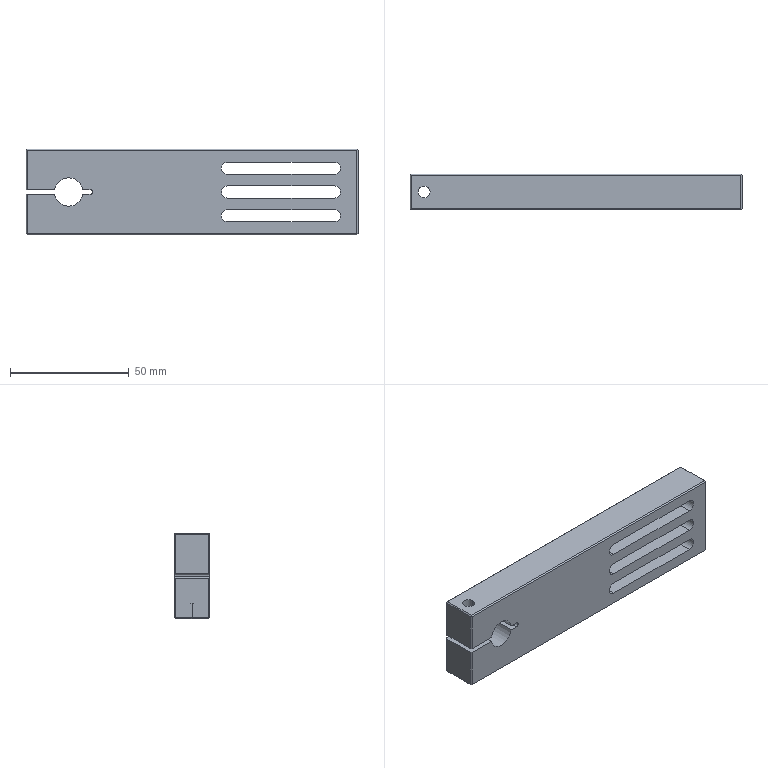Part | STEP file | ND25021-01-JDKM-65-TL | 1 solid | 53 faces | box 140 x 15 x 36 mm | volume 60544 mm3 | plane 36 | cylinder 17 | commonest cylinder face diameters 5.2 x6 12 x3 2 x2 5 x2 6.6 x2 11 x2